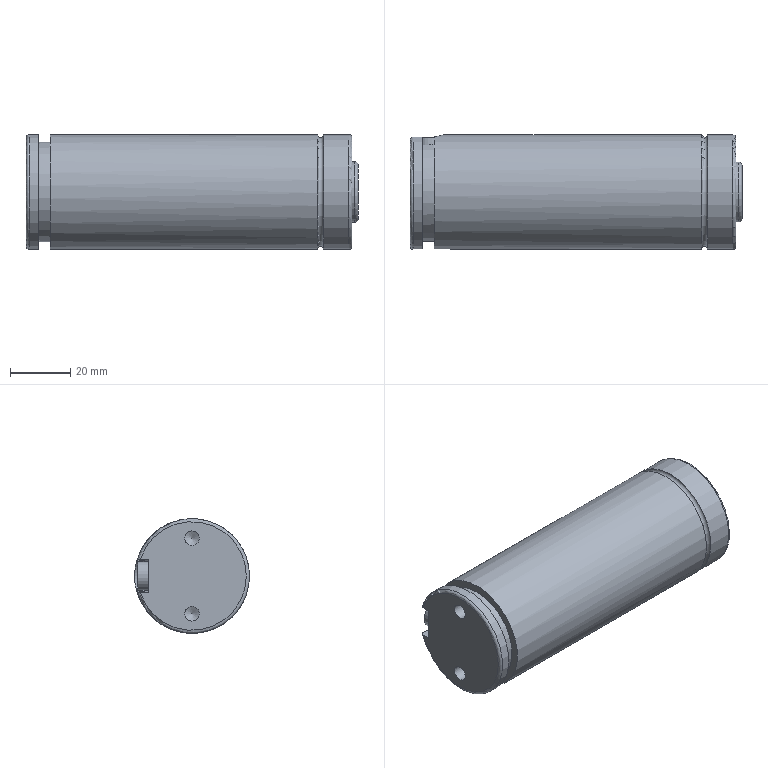Part | NX | features 1 2 | 1 solid | 34 faces | box 110 x 38 x 38 mm | volume 121162 mm3 | plane 16 | cylinder 10 | torus 4 | cone 4 | commonest cylinder face diameters 4.9 x3 38 x3 9.5 x1 11 x1 20 x1 33 x1
STEP:
#1=CARTESIAN_POINT('',(-68.4,-180.,-430.4));
#2=VERTEX_POINT('',#1);
#3=CARTESIAN_POINT('',(-68.4,-180.,-449.4));
#4=DIRECTION('',(-1.,0.,0.));
#5=DIRECTION('',(0.,0.,1.));
#6=AXIS2_PLACEMENT_3D('',#3,#4,#5);
#7=CIRCLE('',#6,19.);
#8=EDGE_CURVE('',#2,#2,#7,.T.);
#9=ORIENTED_EDGE('',*,*,#8,.F.);
#10=EDGE_LOOP('',(#9));
#11=FACE_BOUND('',#10,.T.);
#12=CARTESIAN_POINT('',(-66.4,-180.,-430.4));
#13=VERTEX_POINT('',#12);
#14=CARTESIAN_POINT('',(-66.4,-180.,-449.4));
#15=DIRECTION('',(-1.,0.,0.));
#16=DIRECTION('',(0.,0.,1.));
#17=AXIS2_PLACEMENT_3D('',#14,#15,#16);
#18=CIRCLE('',#17,19.);
#19=EDGE_CURVE('',#13,#13,#18,.T.);
#20=ORIENTED_EDGE('',*,*,#19,.T.);
#21=EDGE_LOOP('',(#20));
#22=FACE_BOUND('',#21,.T.);
#23=CARTESIAN_POINT('',(-67.4,-180.,-449.4));
#24=DIRECTION('',(1.,0.,0.));
#25=DIRECTION('',(0.,-1.,0.));
#26=AXIS2_PLACEMENT_3D('',#23,#24,#25);
#27=TOROIDAL_SURFACE('',#26,19.,1.);
#28=ADVANCED_FACE('',(#11,#22),#27,.F.);
#29=CARTESIAN_POINT('',(-58.,-180.,-430.4));
#30=VERTEX_POINT('',#29);
#31=CARTESIAN_POINT('',(-58.,-180.,-449.4));
#32=DIRECTION('',(-1.,0.,0.));
#33=DIRECTION('',(0.,0.,1.));
#34=AXIS2_PLACEMENT_3D('',#31,#32,#33);
#35=CIRCLE('',#34,19.);
#36=EDGE_CURVE('',#30,#30,#35,.T.);
#37=ORIENTED_EDGE('',*,*,#36,.F.);
#38=EDGE_LOOP('',(#37));
#39=FACE_BOUND('',#38,.T.);
#40=CARTESIAN_POINT('',(-57.,-180.,-431.4));
#41=VERTEX_POINT('',#40);
#42=CARTESIAN_POINT('',(-57.,-180.,-449.4));
#43=DIRECTION('',(-1.,0.,0.));
#44=DIRECTION('',(0.,0.,1.));
#45=AXIS2_PLACEMENT_3D('',#42,#43,#44);
#46=CIRCLE('',#45,18.);
#47=EDGE_CURVE('',#41,#41,#46,.T.);
#48=ORIENTED_EDGE('',*,*,#47,.T.);
#49=EDGE_LOOP('',(#48));
#50=FACE_BOUND('',#49,.T.);
#51=CARTESIAN_POINT('',(-58.,-180.,-449.4));
#52=DIRECTION('',(1.,0.,0.));
#53=DIRECTION('',(0.,-1.,0.));
#54=AXIS2_PLACEMENT_3D('',#51,#52,#53);
#55=TOROIDAL_SURFACE('',#54,18.,1.);
#56=ADVANCED_FACE('',(#39,#50),#55,.T.);
#57=ORIENTED_EDGE('',*,*,#19,.F.);
#58=EDGE_LOOP('',(#57));
#59=FACE_BOUND('',#58,.T.);
#60=ORIENTED_EDGE('',*,*,#36,.T.);
#61=EDGE_LOOP('',(#60));
#62=FACE_BOUND('',#61,.T.);
#63=CARTESIAN_POINT('',(-62.2,-180.,-449.4));
#64=DIRECTION('',(-1.,0.,0.));
#65=DIRECTION('',(0.,1.,0.));
#66=AXIS2_PLACEMENT_3D('',#63,#64,#65);
#67=CYLINDRICAL_SURFACE('',#66,19.);
#68=ADVANCED_FACE('',(#59,#62),#67,.T.);
#69=CARTESIAN_POINT('',(-56.,-180.,-439.4));
#70=VERTEX_POINT('',#69);
#71=CARTESIAN_POINT('',(-56.,-180.,-449.4));
#72=DIRECTION('',(-1.,0.,0.));
#73=DIRECTION('',(0.,0.,1.));
#74=AXIS2_PLACEMENT_3D('',#71,#72,#73);
#75=CIRCLE('',#74,10.);
#76=EDGE_CURVE('',#70,#70,#75,.T.);
#77=ORIENTED_EDGE('',*,*,#76,.F.);
#78=EDGE_LOOP('',(#77));
#79=FACE_BOUND('',#78,.T.);
#80=CARTESIAN_POINT('',(-55.,-180.,-440.4));
#81=VERTEX_POINT('',#80);
#82=CARTESIAN_POINT('',(-55.,-180.,-449.4));
#83=DIRECTION('',(-1.,0.,0.));
#84=DIRECTION('',(0.,0.,1.));
#85=AXIS2_PLACEMENT_3D('',#82,#83,#84);
#86=CIRCLE('',#85,9.);
#87=EDGE_CURVE('',#81,#81,#86,.T.);
#88=ORIENTED_EDGE('',*,*,#87,.T.);
#89=EDGE_LOOP('',(#88));
#90=FACE_BOUND('',#89,.T.);
#91=CARTESIAN_POINT('',(-56.,-180.,-449.4));
#92=DIRECTION('',(1.,0.,0.));
#93=DIRECTION('',(0.,-1.,0.));
#94=AXIS2_PLACEMENT_3D('',#91,#92,#93);
#95=TOROIDAL_SURFACE('',#94,9.,1.);
#96=ADVANCED_FACE('',(#79,#90),#95,.T.);
#97=CARTESIAN_POINT('',(-57.,-180.,-459.4));
#98=VERTEX_POINT('',#97);
#99=CARTESIAN_POINT('',(-57.,-180.,-449.4));
#100=DIRECTION('',(1.,0.,0.));
#101=DIRECTION('',(0.,0.,-1.));
#102=AXIS2_PLACEMENT_3D('',#99,#100,#101);
#103=CIRCLE('',#102,10.);
#104=EDGE_CURVE('',#98,#98,#103,.T.);
#105=ORIENTED_EDGE('',*,*,#104,.T.);
#106=EDGE_LOOP('',(#105));
#107=FACE_BOUND('',#106,.T.);
#108=ORIENTED_EDGE('',*,*,#76,.T.);
#109=EDGE_LOOP('',(#108));
#110=FACE_BOUND('',#109,.T.);
#111=CARTESIAN_POINT('',(46.,-180.,-449.4));
#112=DIRECTION('',(-1.,0.,0.));
#113=DIRECTION('',(0.,1.,0.));
#114=AXIS2_PLACEMENT_3D('',#111,#112,#113);
#115=CYLINDRICAL_SURFACE('',#114,10.);
#116=ADVANCED_FACE('',(#107,#110),#115,.T.);
#117=CARTESIAN_POINT('',(-165.,-180.,-439.35));
#118=VERTEX_POINT('',#117);
#119=CARTESIAN_POINT('',(-165.,-180.,-436.9));
#120=DIRECTION('',(-1.,0.,0.));
#121=DIRECTION('',(0.,0.,-1.));
#122=AXIS2_PLACEMENT_3D('',#119,#120,#121);
#123=CIRCLE('',#122,2.45);
#124=EDGE_CURVE('',#118,#118,#123,.T.);
#125=ORIENTED_EDGE('',*,*,#124,.T.);
#126=EDGE_LOOP('',(#125));
#127=FACE_BOUND('',#126,.T.);
#128=CARTESIAN_POINT('',(-157.8,-180.,-439.35));
#129=VERTEX_POINT('',#128);
#130=CARTESIAN_POINT('',(-157.8,-180.,-436.9));
#131=DIRECTION('',(1.,0.,0.));
#132=DIRECTION('',(0.,0.,-1.));
#133=AXIS2_PLACEMENT_3D('',#130,#131,#132);
#134=CIRCLE('',#133,2.45);
#135=EDGE_CURVE('',#129,#129,#134,.T.);
#136=ORIENTED_EDGE('',*,*,#135,.T.);
#137=EDGE_LOOP('',(#136));
#138=FACE_BOUND('',#137,.T.);
#139=CARTESIAN_POINT('',(-161.4,-180.,-436.9));
#140=DIRECTION('',(1.,0.,0.));
#141=DIRECTION('',(0.,-1.,0.));
#142=AXIS2_PLACEMENT_3D('',#139,#140,#141);
#143=CYLINDRICAL_SURFACE('',#142,2.45);
#144=ADVANCED_FACE('',(#127,#138),#143,.F.);
#145=CARTESIAN_POINT('',(-156.5,-180.,-436.9));
#146=VERTEX_POINT('',#145);
#147=VERTEX_LOOP('',#146);
#148=FACE_BOUND('',#147,.T.);
#149=ORIENTED_EDGE('',*,*,#135,.F.);
#150=EDGE_LOOP('',(#149));
#151=FACE_BOUND('',#150,.T.);
#152=CARTESIAN_POINT('',(-157.15,-180.,-436.9));
#153=DIRECTION('',(-1.,0.,0.));
#154=DIRECTION('',(0.,1.,0.));
#155=AXIS2_PLACEMENT_3D('',#152,#153,#154);
#156=CONICAL_SURFACE('',#155,1.225,1.083);
#157=ADVANCED_FACE('',(#148,#151),#156,.F.);
#158=CARTESIAN_POINT('',(-55.,-180.,-445.9));
#159=VERTEX_POINT('',#158);
#160=CARTESIAN_POINT('',(-55.,-180.,-449.4));
#161=DIRECTION('',(1.,0.,0.));
#162=DIRECTION('',(0.,0.,1.));
#163=AXIS2_PLACEMENT_3D('',#160,#161,#162);
#164=CIRCLE('',#163,3.5);
#165=EDGE_CURVE('',#159,#159,#164,.T.);
#166=ORIENTED_EDGE('',*,*,#165,.T.);
#167=EDGE_LOOP('',(#166));
#168=FACE_BOUND('',#167,.T.);
#169=CARTESIAN_POINT('',(-56.05,-180.,-446.95));
#170=VERTEX_POINT('',#169);
#171=CARTESIAN_POINT('',(-56.05,-180.,-449.4));
#172=DIRECTION('',(-1.,0.,0.));
#173=DIRECTION('',(0.,0.,1.));
#174=AXIS2_PLACEMENT_3D('',#171,#172,#173);
#175=CIRCLE('',#174,2.45);
#176=EDGE_CURVE('',#170,#170,#175,.T.);
#177=ORIENTED_EDGE('',*,*,#176,.T.);
#178=EDGE_LOOP('',(#177));
#179=FACE_BOUND('',#178,.T.);
#180=CARTESIAN_POINT('',(-55.525,-180.,-449.4));
#181=DIRECTION('',(1.,0.,0.));
#182=DIRECTION('',(0.,-1.,0.));
#183=AXIS2_PLACEMENT_3D('',#180,#181,#182);
#184=CONICAL_SURFACE('',#183,2.975,0.7854);
#185=ADVANCED_FACE('',(#168,#179),#184,.F.);
#186=ORIENTED_EDGE('',*,*,#176,.F.);
#187=EDGE_LOOP('',(#186));
#188=FACE_BOUND('',#187,.T.);
#189=CARTESIAN_POINT('',(-61.5,-180.,-446.95));
#190=VERTEX_POINT('',#189);
#191=CARTESIAN_POINT('',(-61.5,-180.,-449.4));
#192=DIRECTION('',(-1.,0.,0.));
#193=DIRECTION('',(0.,0.,1.));
#194=AXIS2_PLACEMENT_3D('',#191,#192,#193);
#195=CIRCLE('',#194,2.45);
#196=EDGE_CURVE('',#190,#190,#195,.T.);
#197=ORIENTED_EDGE('',*,*,#196,.T.);
#198=EDGE_LOOP('',(#197));
#199=FACE_BOUND('',#198,.T.);
#200=CARTESIAN_POINT('',(-58.775,-180.,-449.4));
#201=DIRECTION('',(-1.,0.,0.));
#202=DIRECTION('',(0.,1.,0.));
#203=AXIS2_PLACEMENT_3D('',#200,#201,#202);
#204=CYLINDRICAL_SURFACE('',#203,2.45);
#205=ADVANCED_FACE('',(#188,#199),#204,.F.);
#206=CARTESIAN_POINT('',(-62.5,-180.,-449.4));
#207=VERTEX_POINT('',#206);
#208=VERTEX_LOOP('',#207);
#209=FACE_BOUND('',#208,.T.);
#210=ORIENTED_EDGE('',*,*,#196,.F.);
#211=EDGE_LOOP('',(#210));
#212=FACE_BOUND('',#211,.T.);
#213=CARTESIAN_POINT('',(-62.,-180.,-449.4));
#214=DIRECTION('',(1.,0.,0.));
#215=DIRECTION('',(0.,-1.,0.));
#216=AXIS2_PLACEMENT_3D('',#213,#214,#215);
#217=CONICAL_SURFACE('',#216,1.225,1.183);
#218=ADVANCED_FACE('',(#209,#212),#217,.F.);
#219=CARTESIAN_POINT('',(-157.8,-180.,-459.45));
#220=VERTEX_POINT('',#219);
#221=CARTESIAN_POINT('',(-157.8,-180.,-461.9));
#222=DIRECTION('',(-1.,0.,0.));
#223=DIRECTION('',(0.,0.,1.));
#224=AXIS2_PLACEMENT_3D('',#221,#222,#223);
#225=CIRCLE('',#224,2.45);
#226=EDGE_CURVE('',#220,#220,#225,.T.);
#227=ORIENTED_EDGE('',*,*,#226,.T.);
#228=EDGE_LOOP('',(#227));
#229=FACE_BOUND('',#228,.T.);
#230=CARTESIAN_POINT('',(-156.5,-180.,-461.9));
#231=VERTEX_POINT('',#230);
#232=VERTEX_LOOP('',#231);
#233=FACE_BOUND('',#232,.T.);
#234=CARTESIAN_POINT('',(-157.15,-180.,-461.9));
#235=DIRECTION('',(-1.,0.,0.));
#236=DIRECTION('',(0.,1.,0.));
#237=AXIS2_PLACEMENT_3D('',#234,#235,#236);
#238=CONICAL_SURFACE('',#237,1.225,1.083);
#239=ADVANCED_FACE('',(#229,#233),#238,.F.);
#240=ORIENTED_EDGE('',*,*,#226,.F.);
#241=EDGE_LOOP('',(#240));
#242=FACE_BOUND('',#241,.T.);
#243=CARTESIAN_POINT('',(-165.,-180.,-459.45));
#244=VERTEX_POINT('',#243);
#245=CARTESIAN_POINT('',(-165.,-180.,-461.9));
#246=DIRECTION('',(-1.,0.,0.));
#247=DIRECTION('',(0.,0.,1.));
#248=AXIS2_PLACEMENT_3D('',#245,#246,#247);
#249=CIRCLE('',#248,2.45);
#250=EDGE_CURVE('',#244,#244,#249,.T.);
#251=ORIENTED_EDGE('',*,*,#250,.T.);
#252=EDGE_LOOP('',(#251));
#253=FACE_BOUND('',#252,.T.);
#254=CARTESIAN_POINT('',(-161.4,-180.,-461.9));
#255=DIRECTION('',(-1.,0.,0.));
#256=DIRECTION('',(0.,1.,0.));
#257=AXIS2_PLACEMENT_3D('',#254,#255,#256);
#258=CYLINDRICAL_SURFACE('',#257,2.45);
#259=ADVANCED_FACE('',(#242,#253),#258,.F.);
#260=CARTESIAN_POINT('',(-164.,-161.813,-454.9));
#261=VERTEX_POINT('',#260);
#262=CARTESIAN_POINT('',(-164.,-161.813,-443.9));
#263=VERTEX_POINT('',#262);
#264=CARTESIAN_POINT('',(-164.,-180.,-449.4));
#265=DIRECTION('',(-1.,0.,0.));
#266=DIRECTION('',(0.,0.,1.));
#267=AXIS2_PLACEMENT_3D('',#264,#265,#266);
#268=CIRCLE('',#267,19.);
#269=EDGE_CURVE('',#261,#263,#268,.T.);
#270=ORIENTED_EDGE('',*,*,#269,.F.);
#271=CARTESIAN_POINT('',(-161.,-161.813,-454.9));
#272=VERTEX_POINT('',#271);
#273=CARTESIAN_POINT('',(-162.5,-161.813,-454.9));
#274=DIRECTION('',(-1.,0.,0.));
#275=VECTOR('',#274,1000.);
#276=LINE('',#273,#275);
#277=EDGE_CURVE('',#272,#261,#276,.T.);
#278=ORIENTED_EDGE('',*,*,#277,.F.);
#279=CARTESIAN_POINT('',(-161.,-161.813,-443.9));
#280=VERTEX_POINT('',#279);
#281=CARTESIAN_POINT('',(-161.,-180.,-449.4));
#282=DIRECTION('',(1.,0.,0.));
#283=DIRECTION('',(0.,0.,1.));
#284=AXIS2_PLACEMENT_3D('',#281,#282,#283);
#285=CIRCLE('',#284,19.);
#286=EDGE_CURVE('',#280,#272,#285,.T.);
#287=ORIENTED_EDGE('',*,*,#286,.F.);
#288=CARTESIAN_POINT('',(-162.5,-161.813,-443.9));
#289=DIRECTION('',(1.,0.,0.));
#290=VECTOR('',#289,1000.);
#291=LINE('',#288,#290);
#292=EDGE_CURVE('',#263,#280,#291,.T.);
#293=ORIENTED_EDGE('',*,*,#292,.F.);
#294=EDGE_LOOP('',(#270,#278,#287,#293));
#295=FACE_BOUND('',#294,.T.);
#296=CARTESIAN_POINT('',(-93.7,-180.,-449.4));
#297=DIRECTION('',(-1.,0.,0.));
#298=DIRECTION('',(0.,1.,0.));
#299=AXIS2_PLACEMENT_3D('',#296,#297,#298);
#300=CYLINDRICAL_SURFACE('',#299,19.);
#301=ADVANCED_FACE('',(#295),#300,.T.);
#302=CARTESIAN_POINT('',(-165.,-162.861,-443.9));
#303=VERTEX_POINT('',#302);
#304=CARTESIAN_POINT('',(-165.,-162.861,-443.9));
#305=CARTESIAN_POINT('',(-165.,-162.32,-443.9));
#306=CARTESIAN_POINT('',(-164.542,-161.813,-443.9));
#307=CARTESIAN_POINT('',(-164.,-161.813,-443.9));
#308=B_SPLINE_CURVE_WITH_KNOTS('',3,(#304,#305,#306,#307),.UNSPECIFIED.,.F.,.F.,(4,4),(0.,0.0016),.UNSPECIFIED.);
#309=EDGE_CURVE('',#303,#263,#308,.T.);
#310=ORIENTED_EDGE('',*,*,#309,.F.);
#311=CARTESIAN_POINT('',(-165.,-162.861,-454.9));
#312=VERTEX_POINT('',#311);
#313=CARTESIAN_POINT('',(-165.,-180.,-449.4));
#314=DIRECTION('',(-1.,0.,0.));
#315=DIRECTION('',(0.,0.,1.));
#316=AXIS2_PLACEMENT_3D('',#313,#314,#315);
#317=CIRCLE('',#316,18.);
#318=EDGE_CURVE('',#312,#303,#317,.T.);
#319=ORIENTED_EDGE('',*,*,#318,.F.);
#320=CARTESIAN_POINT('',(-164.,-161.813,-454.9));
#321=CARTESIAN_POINT('',(-164.541,-161.813,-454.9));
#322=CARTESIAN_POINT('',(-165.,-162.32,-454.9));
#323=CARTESIAN_POINT('',(-165.,-162.861,-454.9));
#324=B_SPLINE_CURVE_WITH_KNOTS('',3,(#320,#321,#322,#323),.UNSPECIFIED.,.F.,.F.,(4,4),(0.,0.0016),.UNSPECIFIED.);
#325=EDGE_CURVE('',#261,#312,#324,.T.);
#326=ORIENTED_EDGE('',*,*,#325,.F.);
#327=ORIENTED_EDGE('',*,*,#269,.T.);
#328=EDGE_LOOP('',(#310,#319,#326,#327));
#329=FACE_BOUND('',#328,.T.);
#330=CARTESIAN_POINT('',(-164.,-180.,-449.4));
#331=DIRECTION('',(1.,0.,0.));
#332=DIRECTION('',(0.,-1.,0.));
#333=AXIS2_PLACEMENT_3D('',#330,#331,#332);
#334=TOROIDAL_SURFACE('',#333,18.,1.);
#335=ADVANCED_FACE('',(#329),#334,.T.);
#336=CARTESIAN_POINT('',(-161.,-164.444,-454.9));
#337=VERTEX_POINT('',#336);
#338=CARTESIAN_POINT('',(-161.,-164.444,-443.9));
#339=VERTEX_POINT('',#338);
#340=CARTESIAN_POINT('',(-161.,-180.,-449.4));
#341=DIRECTION('',(-1.,0.,0.));
#342=DIRECTION('',(0.,0.,1.));
#343=AXIS2_PLACEMENT_3D('',#340,#341,#342);
#344=CIRCLE('',#343,16.5);
#345=EDGE_CURVE('',#337,#339,#344,.T.);
#346=ORIENTED_EDGE('',*,*,#345,.F.);
#347=CARTESIAN_POINT('',(-159.,-164.444,-454.9));
#348=VERTEX_POINT('',#347);
#349=CARTESIAN_POINT('',(-160.,-164.444,-454.9));
#350=DIRECTION('',(-1.,0.,0.));
#351=VECTOR('',#350,1000.);
#352=LINE('',#349,#351);
#353=EDGE_CURVE('',#348,#337,#352,.T.);
#354=ORIENTED_EDGE('',*,*,#353,.F.);
#355=CARTESIAN_POINT('',(-157.,-164.316,-454.523));
#356=VERTEX_POINT('',#355);
#357=CARTESIAN_POINT('',(-157.,-164.316,-454.523));
#358=CARTESIAN_POINT('',(-157.641,-164.397,-454.774));
#359=CARTESIAN_POINT('',(-158.307,-164.444,-454.9));
#360=CARTESIAN_POINT('',(-159.,-164.444,-454.9));
#361=B_SPLINE_CURVE_WITH_KNOTS('',3,(#357,#358,#359,#360),.UNSPECIFIED.,.F.,.F.,(4,4),(0.,0.002039),.UNSPECIFIED.);
#362=EDGE_CURVE('',#356,#348,#361,.T.);
#363=ORIENTED_EDGE('',*,*,#362,.F.);
#364=CARTESIAN_POINT('',(-157.,-164.316,-444.277));
#365=VERTEX_POINT('',#364);
#366=CARTESIAN_POINT('',(-157.,-180.,-449.4));
#367=DIRECTION('',(-1.,0.,0.));
#368=DIRECTION('',(0.,0.,1.));
#369=AXIS2_PLACEMENT_3D('',#366,#367,#368);
#370=CIRCLE('',#369,16.5);
#371=EDGE_CURVE('',#356,#365,#370,.T.);
#372=ORIENTED_EDGE('',*,*,#371,.T.);
#373=CARTESIAN_POINT('',(-159.,-164.444,-443.9));
#374=VERTEX_POINT('',#373);
#375=CARTESIAN_POINT('',(-159.,-164.444,-443.9));
#376=CARTESIAN_POINT('',(-158.307,-164.444,-443.9));
#377=CARTESIAN_POINT('',(-157.641,-164.397,-444.026));
#378=CARTESIAN_POINT('',(-157.,-164.316,-444.277));
#379=B_SPLINE_CURVE_WITH_KNOTS('',3,(#375,#376,#377,#378),.UNSPECIFIED.,.F.,.F.,(4,4),(0.,0.002039),.UNSPECIFIED.);
#380=EDGE_CURVE('',#374,#365,#379,.T.);
#381=ORIENTED_EDGE('',*,*,#380,.F.);
#382=CARTESIAN_POINT('',(-160.,-164.444,-443.9));
#383=DIRECTION('',(1.,0.,0.));
#384=VECTOR('',#383,1000.);
#385=LINE('',#382,#384);
#386=EDGE_CURVE('',#339,#374,#385,.T.);
#387=ORIENTED_EDGE('',*,*,#386,.F.);
#388=EDGE_LOOP('',(#346,#354,#363,#372,#381,#387));
#389=FACE_BOUND('',#388,.T.);
#390=CARTESIAN_POINT('',(-159.,-180.,-449.4));
#391=DIRECTION('',(-1.,0.,0.));
#392=DIRECTION('',(0.,1.,0.));
#393=AXIS2_PLACEMENT_3D('',#390,#391,#392);
#394=CYLINDRICAL_SURFACE('',#393,16.5);
#395=ADVANCED_FACE('',(#389),#394,.T.);
#396=CARTESIAN_POINT('',(-157.,-161.704,-444.277));
#397=VERTEX_POINT('',#396);
#398=CARTESIAN_POINT('',(-157.,-161.704,-454.523));
#399=VERTEX_POINT('',#398);
#400=CARTESIAN_POINT('',(-157.,-161.704,-444.277));
#401=CARTESIAN_POINT('',(-155.966,-161.591,-444.68));
#402=CARTESIAN_POINT('',(-154.199,-161.218,-446.083));
#403=CARTESIAN_POINT('',(-153.153,-160.891,-449.402));
#404=CARTESIAN_POINT('',(-154.189,-161.216,-452.7));
#405=CARTESIAN_POINT('',(-155.966,-161.591,-454.12));
#406=CARTESIAN_POINT('',(-157.,-161.704,-454.523));
#407=B_SPLINE_CURVE_WITH_KNOTS('',3,(#400,#401,#402,#403,#404,#405,#406),.UNSPECIFIED.,.F.,.F.,(4,1,1,1,4),(0.,0.003298,0.006596,0.009894,0.01319),.UNSPECIFIED.);
#408=EDGE_CURVE('',#397,#399,#407,.T.);
#409=ORIENTED_EDGE('',*,*,#408,.F.);
#410=CARTESIAN_POINT('',(-157.,-180.,-449.4));
#411=DIRECTION('',(-1.,0.,0.));
#412=DIRECTION('',(0.,0.,1.));
#413=AXIS2_PLACEMENT_3D('',#410,#411,#412);
#414=CIRCLE('',#413,19.);
#415=EDGE_CURVE('',#399,#397,#414,.T.);
#416=ORIENTED_EDGE('',*,*,#415,.F.);
#417=EDGE_LOOP('',(#409,#416));
#418=FACE_BOUND('',#417,.T.);
#419=ORIENTED_EDGE('',*,*,#8,.T.);
#420=EDGE_LOOP('',(#419));
#421=FACE_BOUND('',#420,.T.);
#422=CARTESIAN_POINT('',(-93.7,-180.,-449.4));
#423=DIRECTION('',(-1.,0.,0.));
#424=DIRECTION('',(0.,1.,0.));
#425=AXIS2_PLACEMENT_3D('',#422,#423,#424);
#426=CYLINDRICAL_SURFACE('',#425,19.);
#427=ADVANCED_FACE('',(#418,#421),#426,.T.);
#428=CARTESIAN_POINT('',(-159.,-165.5,-444.65));
#429=VERTEX_POINT('',#428);
#430=CARTESIAN_POINT('',(-159.,-165.5,-449.4));
#431=DIRECTION('',(0.,1.,0.));
#432=DIRECTION('',(0.,0.,1.));
#433=AXIS2_PLACEMENT_3D('',#430,#431,#432);
#434=CIRCLE('',#433,4.75);
#435=EDGE_CURVE('',#429,#429,#434,.T.);
#436=ORIENTED_EDGE('',*,*,#435,.T.);
#437=EDGE_LOOP('',(#436));
#438=FACE_BOUND('',#437,.T.);
#439=CARTESIAN_POINT('',(-159.,-162.,-444.65));
#440=VERTEX_POINT('',#439);
#441=CARTESIAN_POINT('',(-159.,-162.,-449.4));
#442=DIRECTION('',(0.,1.,0.));
#443=DIRECTION('',(0.,0.,1.));
#444=AXIS2_PLACEMENT_3D('',#441,#442,#443);
#445=CIRCLE('',#444,4.75);
#446=EDGE_CURVE('',#440,#440,#445,.T.);
#447=ORIENTED_EDGE('',*,*,#446,.F.);
#448=EDGE_LOOP('',(#447));
#449=FACE_BOUND('',#448,.T.);
#450=CARTESIAN_POINT('',(-159.,-180.,-449.4));
#451=DIRECTION('',(0.,-1.,0.));
#452=DIRECTION('',(0.,0.,1.));
#453=AXIS2_PLACEMENT_3D('',#450,#451,#452);
#454=CYLINDRICAL_SURFACE('',#453,4.75);
#455=ADVANCED_FACE('',(#438,#449),#454,.T.);
#456=CARTESIAN_POINT('',(-159.866,-167.,-447.9));
#457=VERTEX_POINT('',#456);
#458=CARTESIAN_POINT('',(-160.732,-167.,-449.4));
#459=VERTEX_POINT('',#458);
#460=CARTESIAN_POINT('',(-159.866,-167.,-447.9));
#461=DIRECTION('',(-0.5,0.,-0.866));
#462=VECTOR('',#461,1000.);
#463=LINE('',#460,#462);
#464=EDGE_CURVE('',#457,#459,#463,.T.);
#465=ORIENTED_EDGE('',*,*,#464,.T.);
#466=CARTESIAN_POINT('',(-160.732,-162.,-449.4));
#467=VERTEX_POINT('',#466);
#468=CARTESIAN_POINT('',(-160.732,-162.,-449.4));
#469=DIRECTION('',(0.,-1.,0.));
#470=VECTOR('',#469,1000.);
#471=LINE('',#468,#470);
#472=EDGE_CURVE('',#467,#459,#471,.T.);
#473=ORIENTED_EDGE('',*,*,#472,.F.);
#474=CARTESIAN_POINT('',(-159.866,-162.,-447.9));
#475=VERTEX_POINT('',#474);
#476=CARTESIAN_POINT('',(-160.833,-162.,-449.574));
#477=DIRECTION('',(0.5,0.,0.866));
#478=VECTOR('',#477,1000.);
#479=LINE('',#476,#478);
#480=EDGE_CURVE('',#467,#475,#479,.T.);
#481=ORIENTED_EDGE('',*,*,#480,.T.);
#482=CARTESIAN_POINT('',(-159.866,-162.,-447.9));
#483=DIRECTION('',(0.,-1.,0.));
#484=VECTOR('',#483,1000.);
#485=LINE('',#482,#484);
#486=EDGE_CURVE('',#475,#457,#485,.T.);
#487=ORIENTED_EDGE('',*,*,#486,.T.);
#488=EDGE_LOOP('',(#465,#473,#481,#487));
#489=FACE_BOUND('',#488,.T.);
#490=CARTESIAN_POINT('',(-159.866,-162.,-447.9));
#491=DIRECTION('',(-0.866,0.,0.5));
#492=DIRECTION('',(0.5,0.,0.866));
#493=AXIS2_PLACEMENT_3D('',#490,#491,#492);
#494=PLANE('',#493);
#495=ADVANCED_FACE('',(#489),#494,.F.);
#496=CARTESIAN_POINT('',(-159.866,-167.,-450.9));
#497=VERTEX_POINT('',#496);
#498=CARTESIAN_POINT('',(-160.732,-167.,-449.4));
#499=DIRECTION('',(0.5,0.,-0.866));
#500=VECTOR('',#499,1000.);
#501=LINE('',#498,#500);
#502=EDGE_CURVE('',#459,#497,#501,.T.);
#503=ORIENTED_EDGE('',*,*,#502,.T.);
#504=CARTESIAN_POINT('',(-159.866,-162.,-450.9));
#505=VERTEX_POINT('',#504);
#506=CARTESIAN_POINT('',(-159.866,-162.,-450.9));
#507=DIRECTION('',(0.,-1.,0.));
#508=VECTOR('',#507,1000.);
#509=LINE('',#506,#508);
#510=EDGE_CURVE('',#505,#497,#509,.T.);
#511=ORIENTED_EDGE('',*,*,#510,.F.);
#512=CARTESIAN_POINT('',(-161.266,-162.,-448.476));
#513=DIRECTION('',(-0.5,0.,0.866));
#514=VECTOR('',#513,1000.);
#515=LINE('',#512,#514);
#516=EDGE_CURVE('',#505,#467,#515,.T.);
#517=ORIENTED_EDGE('',*,*,#516,.T.);
#518=ORIENTED_EDGE('',*,*,#472,.T.);
#519=EDGE_LOOP('',(#503,#511,#517,#518));
#520=FACE_BOUND('',#519,.T.);
#521=CARTESIAN_POINT('',(-160.732,-162.,-449.4));
#522=DIRECTION('',(-0.866,0.,-0.5));
#523=DIRECTION('',(-0.5,0.,0.866));
#524=AXIS2_PLACEMENT_3D('',#521,#522,#523);
#525=PLANE('',#524);
#526=ADVANCED_FACE('',(#520),#525,.F.);
#527=CARTESIAN_POINT('',(-158.134,-167.,-450.9));
#528=VERTEX_POINT('',#527);
#529=CARTESIAN_POINT('',(-159.866,-167.,-450.9));
#530=DIRECTION('',(1.,0.,0.));
#531=VECTOR('',#530,1000.);
#532=LINE('',#529,#531);
#533=EDGE_CURVE('',#497,#528,#532,.T.);
#534=ORIENTED_EDGE('',*,*,#533,.T.);
#535=CARTESIAN_POINT('',(-158.134,-162.,-450.9));
#536=VERTEX_POINT('',#535);
#537=CARTESIAN_POINT('',(-158.134,-162.,-450.9));
#538=DIRECTION('',(0.,-1.,0.));
#539=VECTOR('',#538,1000.);
#540=LINE('',#537,#539);
#541=EDGE_CURVE('',#536,#528,#540,.T.);
#542=ORIENTED_EDGE('',*,*,#541,.F.);
#543=CARTESIAN_POINT('',(-162.433,-162.,-450.9));
#544=DIRECTION('',(-1.,0.,0.));
#545=VECTOR('',#544,1000.);
#546=LINE('',#543,#545);
#547=EDGE_CURVE('',#536,#505,#546,.T.);
#548=ORIENTED_EDGE('',*,*,#547,.T.);
#549=ORIENTED_EDGE('',*,*,#510,.T.);
#550=EDGE_LOOP('',(#534,#542,#548,#549));
#551=FACE_BOUND('',#550,.T.);
#552=CARTESIAN_POINT('',(-159.866,-162.,-450.9));
#553=DIRECTION('',(0.,0.,-1.));
#554=DIRECTION('',(0.,-1.,0.));
#555=AXIS2_PLACEMENT_3D('',#552,#553,#554);
#556=PLANE('',#555);
#557=ADVANCED_FACE('',(#551),#556,.F.);
#558=CARTESIAN_POINT('',(-157.268,-167.,-449.4));
#559=VERTEX_POINT('',#558);
#560=CARTESIAN_POINT('',(-158.134,-167.,-450.9));
#561=DIRECTION('',(0.5,0.,0.866));
#562=VECTOR('',#561,1000.);
#563=LINE('',#560,#562);
#564=EDGE_CURVE('',#528,#559,#563,.T.);
#565=ORIENTED_EDGE('',*,*,#564,.T.);
#566=CARTESIAN_POINT('',(-157.268,-162.,-449.4));
#567=VERTEX_POINT('',#566);
#568=CARTESIAN_POINT('',(-157.268,-162.,-449.4));
#569=DIRECTION('',(0.,-1.,0.));
#570=VECTOR('',#569,1000.);
#571=LINE('',#568,#570);
#572=EDGE_CURVE('',#567,#559,#571,.T.);
#573=ORIENTED_EDGE('',*,*,#572,.F.);
#574=CARTESIAN_POINT('',(-158.667,-162.,-451.824));
#575=DIRECTION('',(-0.5,0.,-0.866));
#576=VECTOR('',#575,1000.);
#577=LINE('',#574,#576);
#578=EDGE_CURVE('',#567,#536,#577,.T.);
#579=ORIENTED_EDGE('',*,*,#578,.T.);
#580=ORIENTED_EDGE('',*,*,#541,.T.);
#581=EDGE_LOOP('',(#565,#573,#579,#580));
#582=FACE_BOUND('',#581,.T.);
#583=CARTESIAN_POINT('',(-158.134,-162.,-450.9));
#584=DIRECTION('',(0.866,0.,-0.5));
#585=DIRECTION('',(-0.5,0.,-0.866));
#586=AXIS2_PLACEMENT_3D('',#583,#584,#585);
#587=PLANE('',#586);
#588=ADVANCED_FACE('',(#582),#587,.F.);
#589=CARTESIAN_POINT('',(-158.134,-167.,-447.9));
#590=VERTEX_POINT('',#589);
#591=CARTESIAN_POINT('',(-157.268,-167.,-449.4));
#592=DIRECTION('',(-0.5,0.,0.866));
#593=VECTOR('',#592,1000.);
#594=LINE('',#591,#593);
#595=EDGE_CURVE('',#559,#590,#594,.T.);
#596=ORIENTED_EDGE('',*,*,#595,.T.);
#597=CARTESIAN_POINT('',(-158.134,-162.,-447.9));
#598=VERTEX_POINT('',#597);
#599=CARTESIAN_POINT('',(-158.134,-162.,-447.9));
#600=DIRECTION('',(0.,-1.,0.));
#601=VECTOR('',#600,1000.);
#602=LINE('',#599,#601);
#603=EDGE_CURVE('',#598,#590,#602,.T.);
#604=ORIENTED_EDGE('',*,*,#603,.F.);
#605=CARTESIAN_POINT('',(-158.234,-162.,-447.726));
#606=DIRECTION('',(0.5,0.,-0.866));
#607=VECTOR('',#606,1000.);
#608=LINE('',#605,#607);
#609=EDGE_CURVE('',#598,#567,#608,.T.);
#610=ORIENTED_EDGE('',*,*,#609,.T.);
#611=ORIENTED_EDGE('',*,*,#572,.T.);
#612=EDGE_LOOP('',(#596,#604,#610,#611));
#613=FACE_BOUND('',#612,.T.);
#614=CARTESIAN_POINT('',(-157.268,-162.,-449.4));
#615=DIRECTION('',(0.866,0.,0.5));
#616=DIRECTION('',(0.5,0.,-0.866));
#617=AXIS2_PLACEMENT_3D('',#614,#615,#616);
#618=PLANE('',#617);
#619=ADVANCED_FACE('',(#613),#618,.F.);
#620=CARTESIAN_POINT('',(-158.134,-167.,-447.9));
#621=DIRECTION('',(-1.,0.,0.));
#622=VECTOR('',#621,1000.);
#623=LINE('',#620,#622);
#624=EDGE_CURVE('',#590,#457,#623,.T.);
#625=ORIENTED_EDGE('',*,*,#624,.T.);
#626=ORIENTED_EDGE('',*,*,#486,.F.);
#627=CARTESIAN_POINT('',(-161.567,-162.,-447.9));
#628=DIRECTION('',(1.,0.,0.));
#629=VECTOR('',#628,1000.);
#630=LINE('',#627,#629);
#631=EDGE_CURVE('',#475,#598,#630,.T.);
#632=ORIENTED_EDGE('',*,*,#631,.T.);
#633=ORIENTED_EDGE('',*,*,#603,.T.);
#634=EDGE_LOOP('',(#625,#626,#632,#633));
#635=FACE_BOUND('',#634,.T.);
#636=CARTESIAN_POINT('',(-158.134,-162.,-447.9));
#637=DIRECTION('',(0.,0.,1.));
#638=DIRECTION('',(0.,1.,0.));
#639=AXIS2_PLACEMENT_3D('',#636,#637,#638);
#640=PLANE('',#639);
#641=ADVANCED_FACE('',(#635),#640,.F.);
#642=ORIENTED_EDGE('',*,*,#464,.F.);
#643=ORIENTED_EDGE('',*,*,#624,.F.);
#644=ORIENTED_EDGE('',*,*,#595,.F.);
#645=ORIENTED_EDGE('',*,*,#564,.F.);
#646=ORIENTED_EDGE('',*,*,#533,.F.);
#647=ORIENTED_EDGE('',*,*,#502,.F.);
#648=EDGE_LOOP('',(#642,#643,#644,#645,#646,#647));
#649=FACE_BOUND('',#648,.T.);
#650=CARTESIAN_POINT('',(-159.,-167.,-449.4));
#651=DIRECTION('',(0.,1.,0.));
#652=DIRECTION('',(0.,0.,-1.));
#653=AXIS2_PLACEMENT_3D('',#650,#651,#652);
#654=PLANE('',#653);
#655=ADVANCED_FACE('',(#649),#654,.T.);
#656=ORIENTED_EDGE('',*,*,#480,.F.);
#657=ORIENTED_EDGE('',*,*,#516,.F.);
#658=ORIENTED_EDGE('',*,*,#547,.F.);
#659=ORIENTED_EDGE('',*,*,#578,.F.);
#660=ORIENTED_EDGE('',*,*,#609,.F.);
#661=ORIENTED_EDGE('',*,*,#631,.F.);
#662=EDGE_LOOP('',(#656,#657,#658,#659,#660,#661));
#663=FACE_BOUND('',#662,.T.);
#664=ORIENTED_EDGE('',*,*,#446,.T.);
#665=EDGE_LOOP('',(#664));
#666=FACE_BOUND('',#665,.T.);
#667=CARTESIAN_POINT('',(-165.,-162.,-449.4));
#668=DIRECTION('',(0.,-1.,0.));
#669=DIRECTION('',(0.,0.,1.));
#670=AXIS2_PLACEMENT_3D('',#667,#668,#669);
#671=PLANE('',#670);
#672=ADVANCED_FACE('',(#663,#666),#671,.F.);
#673=ORIENTED_EDGE('',*,*,#362,.T.);
#674=CARTESIAN_POINT('',(-159.,-165.5,-454.9));
#675=VERTEX_POINT('',#674);
#676=CARTESIAN_POINT('',(-159.,-161.,-454.9));
#677=DIRECTION('',(0.,-1.,0.));
#678=VECTOR('',#677,1000.);
#679=LINE('',#676,#678);
#680=EDGE_CURVE('',#348,#675,#679,.T.);
#681=ORIENTED_EDGE('',*,*,#680,.T.);
#682=CARTESIAN_POINT('',(-159.,-165.5,-443.9));
#683=VERTEX_POINT('',#682);
#684=CARTESIAN_POINT('',(-159.,-165.5,-449.4));
#685=DIRECTION('',(0.,-1.,0.));
#686=DIRECTION('',(0.,0.,1.));
#687=AXIS2_PLACEMENT_3D('',#684,#685,#686);
#688=CIRCLE('',#687,5.5);
#689=EDGE_CURVE('',#675,#683,#688,.T.);
#690=ORIENTED_EDGE('',*,*,#689,.T.);
#691=CARTESIAN_POINT('',(-159.,-161.,-443.9));
#692=DIRECTION('',(0.,-1.,0.));
#693=VECTOR('',#692,1000.);
#694=LINE('',#691,#693);
#695=EDGE_CURVE('',#374,#683,#694,.T.);
#696=ORIENTED_EDGE('',*,*,#695,.F.);
#697=ORIENTED_EDGE('',*,*,#380,.T.);
#698=CARTESIAN_POINT('',(-157.,-163.25,-444.277));
#699=DIRECTION('',(0.,1.,0.));
#700=VECTOR('',#699,1000.);
#701=LINE('',#698,#700);
#702=EDGE_CURVE('',#365,#397,#701,.T.);
#703=ORIENTED_EDGE('',*,*,#702,.T.);
#704=ORIENTED_EDGE('',*,*,#408,.T.);
#705=CARTESIAN_POINT('',(-157.,-163.25,-454.523));
#706=DIRECTION('',(0.,-1.,0.));
#707=VECTOR('',#706,1000.);
#708=LINE('',#705,#707);
#709=EDGE_CURVE('',#399,#356,#708,.T.);
#710=ORIENTED_EDGE('',*,*,#709,.T.);
#711=EDGE_LOOP('',(#673,#681,#690,#696,#697,#703,#704,#710));
#712=FACE_BOUND('',#711,.T.);
#713=CARTESIAN_POINT('',(-159.,-161.,-449.4));
#714=DIRECTION('',(0.,1.,0.));
#715=DIRECTION('',(0.,0.,-1.));
#716=AXIS2_PLACEMENT_3D('',#713,#714,#715);
#717=CYLINDRICAL_SURFACE('',#716,5.5);
#718=ADVANCED_FACE('',(#712),#717,.F.);
#719=ORIENTED_EDGE('',*,*,#353,.T.);
#720=CARTESIAN_POINT('',(-161.,-170.5,-454.9));
#721=DIRECTION('',(0.,1.,0.));
#722=VECTOR('',#721,1000.);
#723=LINE('',#720,#722);
#724=EDGE_CURVE('',#337,#272,#723,.T.);
#725=ORIENTED_EDGE('',*,*,#724,.T.);
#726=ORIENTED_EDGE('',*,*,#277,.T.);
#727=ORIENTED_EDGE('',*,*,#325,.T.);
#728=CARTESIAN_POINT('',(-165.,-165.5,-454.9));
#729=VERTEX_POINT('',#728);
#730=CARTESIAN_POINT('',(-165.,-170.5,-454.9));
#731=DIRECTION('',(0.,-1.,0.));
#732=VECTOR('',#731,1000.);
#733=LINE('',#730,#732);
#734=EDGE_CURVE('',#312,#729,#733,.T.);
#735=ORIENTED_EDGE('',*,*,#734,.T.);
#736=CARTESIAN_POINT('',(-159.,-165.5,-454.9));
#737=DIRECTION('',(1.,0.,0.));
#738=VECTOR('',#737,1000.);
#739=LINE('',#736,#738);
#740=EDGE_CURVE('',#729,#675,#739,.T.);
#741=ORIENTED_EDGE('',*,*,#740,.T.);
#742=ORIENTED_EDGE('',*,*,#680,.F.);
#743=EDGE_LOOP('',(#719,#725,#726,#727,#735,#741,#742));
#744=FACE_BOUND('',#743,.T.);
#745=CARTESIAN_POINT('',(-165.,-161.,-454.9));
#746=DIRECTION('',(0.,0.,-1.));
#747=DIRECTION('',(0.,-1.,0.));
#748=AXIS2_PLACEMENT_3D('',#745,#746,#747);
#749=PLANE('',#748);
#750=ADVANCED_FACE('',(#744),#749,.F.);
#751=ORIENTED_EDGE('',*,*,#386,.T.);
#752=ORIENTED_EDGE('',*,*,#695,.T.);
#753=CARTESIAN_POINT('',(-165.,-165.5,-443.9));
#754=VERTEX_POINT('',#753);
#755=CARTESIAN_POINT('',(-165.,-165.5,-443.9));
#756=DIRECTION('',(-1.,0.,0.));
#757=VECTOR('',#756,1000.);
#758=LINE('',#755,#757);
#759=EDGE_CURVE('',#683,#754,#758,.T.);
#760=ORIENTED_EDGE('',*,*,#759,.T.);
#761=CARTESIAN_POINT('',(-165.,-170.5,-443.9));
#762=DIRECTION('',(0.,1.,0.));
#763=VECTOR('',#762,1000.);
#764=LINE('',#761,#763);
#765=EDGE_CURVE('',#754,#303,#764,.T.);
#766=ORIENTED_EDGE('',*,*,#765,.T.);
#767=ORIENTED_EDGE('',*,*,#309,.T.);
#768=ORIENTED_EDGE('',*,*,#292,.T.);
#769=CARTESIAN_POINT('',(-161.,-170.5,-443.9));
#770=DIRECTION('',(0.,-1.,0.));
#771=VECTOR('',#770,1000.);
#772=LINE('',#769,#771);
#773=EDGE_CURVE('',#280,#339,#772,.T.);
#774=ORIENTED_EDGE('',*,*,#773,.T.);
#775=EDGE_LOOP('',(#751,#752,#760,#766,#767,#768,#774));
#776=FACE_BOUND('',#775,.T.);
#777=CARTESIAN_POINT('',(-159.,-161.,-443.9));
#778=DIRECTION('',(0.,0.,1.));
#779=DIRECTION('',(0.,1.,0.));
#780=AXIS2_PLACEMENT_3D('',#777,#778,#779);
#781=PLANE('',#780);
#782=ADVANCED_FACE('',(#776),#781,.F.);
#783=ORIENTED_EDGE('',*,*,#435,.F.);
#784=EDGE_LOOP('',(#783));
#785=FACE_BOUND('',#784,.T.);
#786=ORIENTED_EDGE('',*,*,#740,.F.);
#787=CARTESIAN_POINT('',(-165.,-165.5,-444.9));
#788=DIRECTION('',(0.,0.,1.));
#789=VECTOR('',#788,1000.);
#790=LINE('',#787,#789);
#791=EDGE_CURVE('',#729,#754,#790,.T.);
#792=ORIENTED_EDGE('',*,*,#791,.T.);
#793=ORIENTED_EDGE('',*,*,#759,.F.);
#794=ORIENTED_EDGE('',*,*,#689,.F.);
#795=EDGE_LOOP('',(#786,#792,#793,#794));
#796=FACE_BOUND('',#795,.T.);
#797=CARTESIAN_POINT('',(-165.,-165.5,-449.4));
#798=DIRECTION('',(0.,-1.,0.));
#799=DIRECTION('',(0.,0.,1.));
#800=AXIS2_PLACEMENT_3D('',#797,#798,#799);
#801=PLANE('',#800);
#802=ADVANCED_FACE('',(#785,#796),#801,.F.);
#803=ORIENTED_EDGE('',*,*,#709,.F.);
#804=ORIENTED_EDGE('',*,*,#415,.T.);
#805=ORIENTED_EDGE('',*,*,#702,.F.);
#806=ORIENTED_EDGE('',*,*,#371,.F.);
#807=EDGE_LOOP('',(#803,#804,#805,#806));
#808=FACE_BOUND('',#807,.T.);
#809=CARTESIAN_POINT('',(-157.,-180.,-431.55));
#810=DIRECTION('',(1.,0.,0.));
#811=DIRECTION('',(0.,-1.,0.));
#812=AXIS2_PLACEMENT_3D('',#809,#810,#811);
#813=PLANE('',#812);
#814=ADVANCED_FACE('',(#808),#813,.F.);
#815=ORIENTED_EDGE('',*,*,#724,.F.);
#816=ORIENTED_EDGE('',*,*,#345,.T.);
#817=ORIENTED_EDGE('',*,*,#773,.F.);
#818=ORIENTED_EDGE('',*,*,#286,.T.);
#819=EDGE_LOOP('',(#815,#816,#817,#818));
#820=FACE_BOUND('',#819,.T.);
#821=CARTESIAN_POINT('',(-161.,-180.,-431.55));
#822=DIRECTION('',(-1.,0.,0.));
#823=DIRECTION('',(0.,1.,0.));
#824=AXIS2_PLACEMENT_3D('',#821,#822,#823);
#825=PLANE('',#824);
#826=ADVANCED_FACE('',(#820),#825,.F.);
#827=ORIENTED_EDGE('',*,*,#734,.F.);
#828=ORIENTED_EDGE('',*,*,#318,.T.);
#829=ORIENTED_EDGE('',*,*,#765,.F.);
#830=ORIENTED_EDGE('',*,*,#791,.F.);
#831=EDGE_LOOP('',(#827,#828,#829,#830));
#832=FACE_BOUND('',#831,.T.);
#833=ORIENTED_EDGE('',*,*,#124,.F.);
#834=EDGE_LOOP('',(#833));
#835=FACE_BOUND('',#834,.T.);
#836=ORIENTED_EDGE('',*,*,#250,.F.);
#837=EDGE_LOOP('',(#836));
#838=FACE_BOUND('',#837,.T.);
#839=CARTESIAN_POINT('',(-165.,-180.,-440.4));
#840=DIRECTION('',(-1.,0.,0.));
#841=DIRECTION('',(0.,0.,1.));
#842=AXIS2_PLACEMENT_3D('',#839,#840,#841);
#843=PLANE('',#842);
#844=ADVANCED_FACE('',(#832,#835,#838),#843,.T.);
#845=ORIENTED_EDGE('',*,*,#165,.F.);
#846=EDGE_LOOP('',(#845));
#847=FACE_BOUND('',#846,.T.);
#848=ORIENTED_EDGE('',*,*,#87,.F.);
#849=EDGE_LOOP('',(#848));
#850=FACE_BOUND('',#849,.T.);
#851=CARTESIAN_POINT('',(-55.,-180.,-444.9));
#852=DIRECTION('',(1.,0.,0.));
#853=DIRECTION('',(0.,-1.,0.));
#854=AXIS2_PLACEMENT_3D('',#851,#852,#853);
#855=PLANE('',#854);
#856=ADVANCED_FACE('',(#847,#850),#855,.T.);
#857=ORIENTED_EDGE('',*,*,#104,.F.);
#858=EDGE_LOOP('',(#857));
#859=FACE_BOUND('',#858,.T.);
#860=ORIENTED_EDGE('',*,*,#47,.F.);
#861=EDGE_LOOP('',(#860));
#862=FACE_BOUND('',#861,.T.);
#863=CARTESIAN_POINT('',(-57.,-180.,-440.4));
#864=DIRECTION('',(1.,0.,0.));
#865=DIRECTION('',(0.,-1.,0.));
#866=AXIS2_PLACEMENT_3D('',#863,#864,#865);
#867=PLANE('',#866);
#868=ADVANCED_FACE('',(#859,#862),#867,.T.);
#869=CLOSED_SHELL('',(#28,#56,#68,#96,#116,#144,#157,#185,#205,#218,#239,#259,#301,#335,#395,#427,#455,#495,#526,#557,#588,#619,#641,#655,#672,#718,#750,#782,#802,#814,#826,#844,#856,#868));
#870=MANIFOLD_SOLID_BREP('',#869);
#871=(LENGTH_UNIT()NAMED_UNIT(*)SI_UNIT(.MILLI.,.METRE.));
#872=UNCERTAINTY_MEASURE_WITH_UNIT(LENGTH_MEASURE(0.0508),#871,'','');
#873=(NAMED_UNIT(*)PLANE_ANGLE_UNIT()SI_UNIT($,.RADIAN.));
#874=(NAMED_UNIT(*)SI_UNIT($,.STERADIAN.)SOLID_ANGLE_UNIT());
#875=(GEOMETRIC_REPRESENTATION_CONTEXT(3)GLOBAL_UNCERTAINTY_ASSIGNED_CONTEXT((#872))GLOBAL_UNIT_ASSIGNED_CONTEXT((#871,#873,#874))REPRESENTATION_CONTEXT('',''));
#876=ADVANCED_BREP_SHAPE_REPRESENTATION('',(#870),#875);